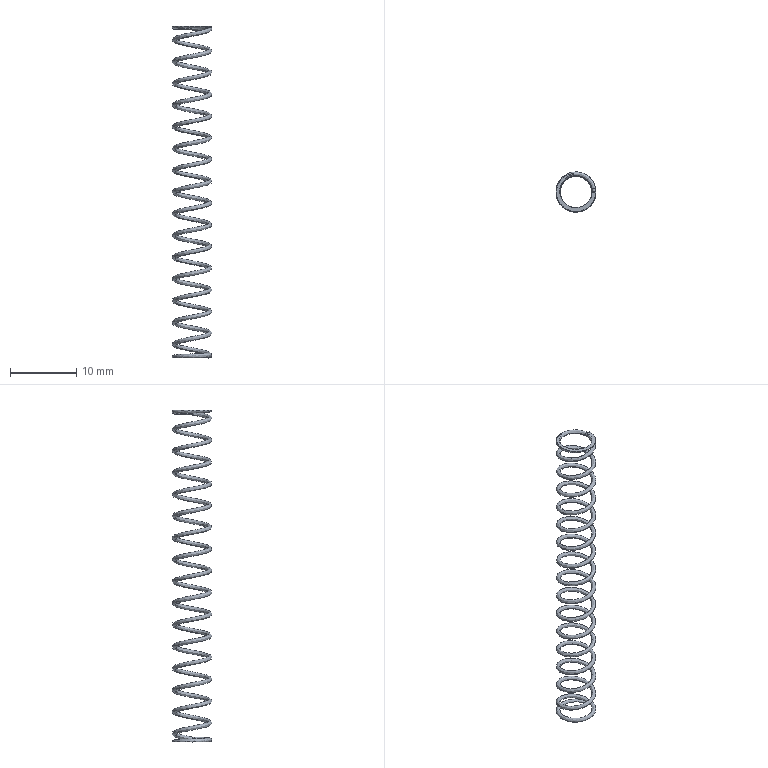Part | STEP file | 1 solid | 9 faces | box 5.998 x 5.997 x 50.45 mm | volume 77.124 mm3 | spline 5 | plane 4